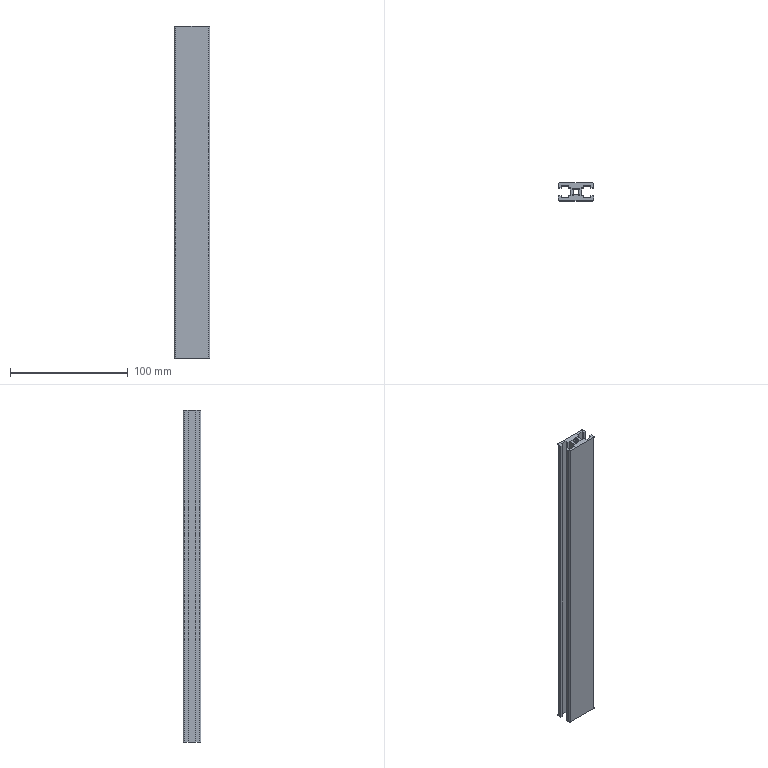Part | NX | features BREP 1 | 1 solid | 99 faces | box 30 x 15 x 282 mm | volume 67389 mm3 | plane 54 | cylinder 41 | cone 4 | commonest cylinder face diameters 1 x18 5 x15 2 x4 6.8 x4